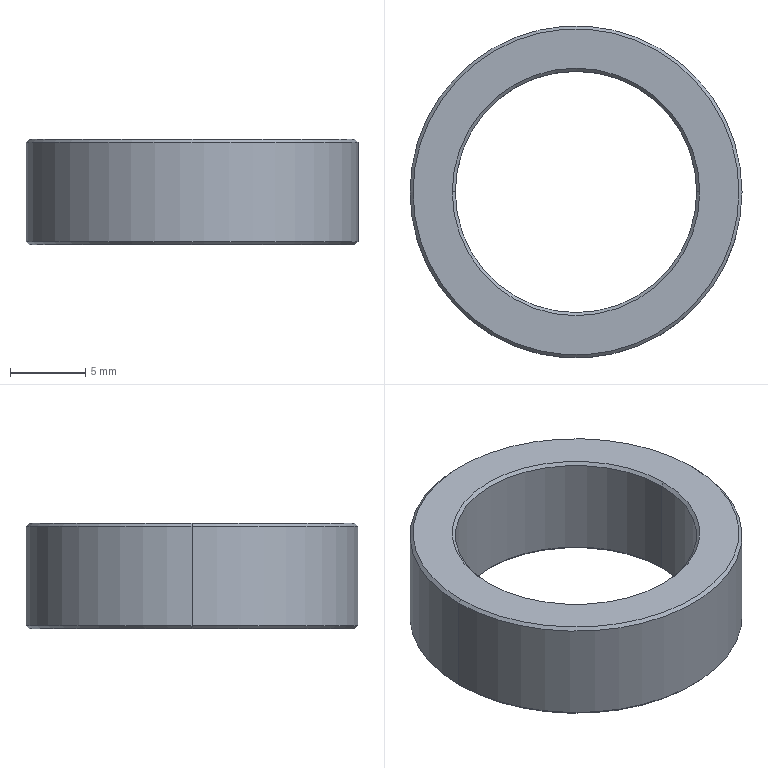Part | STEP file | BPSP-03-037Lift Retaining Ring_Default | 1 solid | 14 faces | box 22 x 22 x 7 mm | volume 1249 mm3 | cone 8 | cylinder 4 | plane 2 | commonest cylinder face diameters 16 x2 22 x2
STEP:
#1=CARTESIAN_POINT('',(0.,0.,0.));
#2=DIRECTION('',(0.,0.,1.));
#3=DIRECTION('',(1.,0.,0.));
#4=AXIS2_PLACEMENT_3D('',#1,#2,#3);
#5=CARTESIAN_POINT('',(10.8,0.,3.5));
#6=VERTEX_POINT('',#5);
#7=CARTESIAN_POINT('',(-10.8,0.,3.5));
#8=VERTEX_POINT('',#7);
#9=CARTESIAN_POINT('',(0.,0.,3.5));
#10=DIRECTION('',(0.,0.,1.));
#11=DIRECTION('',(1.,0.,0.));
#12=AXIS2_PLACEMENT_3D('',#9,#10,#11);
#13=CIRCLE('',#12,10.8);
#14=CARTESIAN_POINT('',(0.,0.,3.5));
#15=DIRECTION('',(0.,0.,-1.));
#16=DIRECTION('',(-1.,0.,0.));
#17=AXIS2_PLACEMENT_3D('',#14,#15,#16);
#18=CONICAL_SURFACE('',#17,10.8,0.7854);
#19=CARTESIAN_POINT('',(3.142,0.));
#20=DIRECTION('',(-1.,0.));
#21=VECTOR('',#20,1.);
#22=LINE('',#19,#21);
#23=(GEOMETRIC_REPRESENTATION_CONTEXT(2)PARAMETRIC_REPRESENTATION_CONTEXT()REPRESENTATION_CONTEXT('',''));
#24=DEFINITIONAL_REPRESENTATION('',(#22),#23);
#25=PCURVE('',#18,#24);
#26=CARTESIAN_POINT('',(0.,0.,3.5));
#27=DIRECTION('',(0.,0.,1.));
#28=DIRECTION('',(1.,0.,0.));
#29=AXIS2_PLACEMENT_3D('',#26,#27,#28);
#30=PLANE('',#29);
#31=CARTESIAN_POINT('',(0.,0.));
#32=DIRECTION('',(1.,0.));
#33=AXIS2_PLACEMENT_2D('',#31,#32);
#34=CIRCLE('',#33,10.8);
#35=(GEOMETRIC_REPRESENTATION_CONTEXT(2)PARAMETRIC_REPRESENTATION_CONTEXT()REPRESENTATION_CONTEXT('',''));
#36=DEFINITIONAL_REPRESENTATION('',(#34),#35);
#37=PCURVE('',#30,#36);
#38=SURFACE_CURVE('',#13,(#25,#37),.PCURVE_S1.);
#39=EDGE_CURVE('',#6,#8,#38,.T.);
#40=ORIENTED_EDGE('',*,*,#39,.F.);
#41=CARTESIAN_POINT('',(11.,0.,3.3));
#42=VERTEX_POINT('',#41);
#43=CARTESIAN_POINT('',(10.8,0.,3.5));
#44=DIRECTION('',(0.7071,0.,-0.7071));
#45=VECTOR('',#44,1.);
#46=LINE('',#43,#45);
#47=CARTESIAN_POINT('',(3.142,0.));
#48=DIRECTION('',(0.,1.));
#49=VECTOR('',#48,1.);
#50=LINE('',#47,#49);
#51=(GEOMETRIC_REPRESENTATION_CONTEXT(2)PARAMETRIC_REPRESENTATION_CONTEXT()REPRESENTATION_CONTEXT('',''));
#52=DEFINITIONAL_REPRESENTATION('',(#50),#51);
#53=PCURVE('',#18,#52);
#54=CARTESIAN_POINT('',(0.,0.,3.5));
#55=DIRECTION('',(0.,0.,-1.));
#56=DIRECTION('',(-1.,0.,0.));
#57=AXIS2_PLACEMENT_3D('',#54,#55,#56);
#58=CONICAL_SURFACE('',#57,10.8,0.7854);
#59=CARTESIAN_POINT('',(3.142,0.));
#60=DIRECTION('',(0.,1.));
#61=VECTOR('',#60,1.);
#62=LINE('',#59,#61);
#63=(GEOMETRIC_REPRESENTATION_CONTEXT(2)PARAMETRIC_REPRESENTATION_CONTEXT()REPRESENTATION_CONTEXT('',''));
#64=DEFINITIONAL_REPRESENTATION('',(#62),#63);
#65=PCURVE('',#58,#64);
#66=SURFACE_CURVE('',#46,(#53,#65),.PCURVE_S1.);
#67=EDGE_CURVE('',#6,#42,#66,.T.);
#68=ORIENTED_EDGE('',*,*,#67,.T.);
#69=CARTESIAN_POINT('',(-11.,0.,3.3));
#70=VERTEX_POINT('',#69);
#71=CARTESIAN_POINT('',(0.,0.,3.3));
#72=DIRECTION('',(0.,0.,-1.));
#73=DIRECTION('',(1.,0.,0.));
#74=AXIS2_PLACEMENT_3D('',#71,#72,#73);
#75=CIRCLE('',#74,11.);
#76=CARTESIAN_POINT('',(-3.142,0.2));
#77=DIRECTION('',(1.,0.));
#78=VECTOR('',#77,1.);
#79=LINE('',#76,#78);
#80=(GEOMETRIC_REPRESENTATION_CONTEXT(2)PARAMETRIC_REPRESENTATION_CONTEXT()REPRESENTATION_CONTEXT('',''));
#81=DEFINITIONAL_REPRESENTATION('',(#79),#80);
#82=PCURVE('',#18,#81);
#83=CARTESIAN_POINT('',(0.,0.,3.5));
#84=DIRECTION('',(0.,0.,-1.));
#85=DIRECTION('',(-1.,0.,0.));
#86=AXIS2_PLACEMENT_3D('',#83,#84,#85);
#87=CYLINDRICAL_SURFACE('',#86,11.);
#88=CARTESIAN_POINT('',(-3.142,0.2));
#89=DIRECTION('',(1.,0.));
#90=VECTOR('',#89,1.);
#91=LINE('',#88,#90);
#92=(GEOMETRIC_REPRESENTATION_CONTEXT(2)PARAMETRIC_REPRESENTATION_CONTEXT()REPRESENTATION_CONTEXT('',''));
#93=DEFINITIONAL_REPRESENTATION('',(#91),#92);
#94=PCURVE('',#87,#93);
#95=SURFACE_CURVE('',#75,(#82,#94),.PCURVE_S1.);
#96=EDGE_CURVE('',#70,#42,#95,.T.);
#97=ORIENTED_EDGE('',*,*,#96,.F.);
#98=CARTESIAN_POINT('',(-10.8,0.,3.5));
#99=DIRECTION('',(-0.7071,0.,-0.7071));
#100=VECTOR('',#99,1.);
#101=LINE('',#98,#100);
#102=CARTESIAN_POINT('',(0.,0.));
#103=DIRECTION('',(0.,1.));
#104=VECTOR('',#103,1.);
#105=LINE('',#102,#104);
#106=(GEOMETRIC_REPRESENTATION_CONTEXT(2)PARAMETRIC_REPRESENTATION_CONTEXT()REPRESENTATION_CONTEXT('',''));
#107=DEFINITIONAL_REPRESENTATION('',(#105),#106);
#108=PCURVE('',#18,#107);
#109=CARTESIAN_POINT('',(6.283,0.));
#110=DIRECTION('',(0.,1.));
#111=VECTOR('',#110,1.);
#112=LINE('',#109,#111);
#113=(GEOMETRIC_REPRESENTATION_CONTEXT(2)PARAMETRIC_REPRESENTATION_CONTEXT()REPRESENTATION_CONTEXT('',''));
#114=DEFINITIONAL_REPRESENTATION('',(#112),#113);
#115=PCURVE('',#58,#114);
#116=SURFACE_CURVE('',#101,(#108,#115),.PCURVE_S1.);
#117=EDGE_CURVE('',#8,#70,#116,.T.);
#118=ORIENTED_EDGE('',*,*,#117,.F.);
#119=EDGE_LOOP('',(#40,#68,#97,#118));
#120=FACE_BOUND('',#119,.T.);
#121=ADVANCED_FACE('',(#120),#18,.T.);
#122=CARTESIAN_POINT('',(8.,0.,3.3));
#123=VERTEX_POINT('',#122);
#124=CARTESIAN_POINT('',(8.2,0.,3.5));
#125=VERTEX_POINT('',#124);
#126=CARTESIAN_POINT('',(8.,0.,3.3));
#127=DIRECTION('',(0.7071,0.,0.7071));
#128=VECTOR('',#127,1.);
#129=LINE('',#126,#128);
#130=CARTESIAN_POINT('',(0.,0.,3.3));
#131=DIRECTION('',(0.,0.,1.));
#132=DIRECTION('',(1.,0.,0.));
#133=AXIS2_PLACEMENT_3D('',#130,#131,#132);
#134=CONICAL_SURFACE('',#133,8.,0.7854);
#135=CARTESIAN_POINT('',(6.283,0.));
#136=DIRECTION('',(0.,1.));
#137=VECTOR('',#136,1.);
#138=LINE('',#135,#137);
#139=(GEOMETRIC_REPRESENTATION_CONTEXT(2)PARAMETRIC_REPRESENTATION_CONTEXT()REPRESENTATION_CONTEXT('',''));
#140=DEFINITIONAL_REPRESENTATION('',(#138),#139);
#141=PCURVE('',#134,#140);
#142=CARTESIAN_POINT('',(0.,0.,3.3));
#143=DIRECTION('',(0.,0.,1.));
#144=DIRECTION('',(1.,0.,0.));
#145=AXIS2_PLACEMENT_3D('',#142,#143,#144);
#146=CONICAL_SURFACE('',#145,8.,0.7854);
#147=CARTESIAN_POINT('',(0.,0.));
#148=DIRECTION('',(0.,1.));
#149=VECTOR('',#148,1.);
#150=LINE('',#147,#149);
#151=(GEOMETRIC_REPRESENTATION_CONTEXT(2)PARAMETRIC_REPRESENTATION_CONTEXT()REPRESENTATION_CONTEXT('',''));
#152=DEFINITIONAL_REPRESENTATION('',(#150),#151);
#153=PCURVE('',#146,#152);
#154=SURFACE_CURVE('',#129,(#141,#153),.PCURVE_S1.);
#155=EDGE_CURVE('',#123,#125,#154,.T.);
#156=ORIENTED_EDGE('',*,*,#155,.T.);
#157=CARTESIAN_POINT('',(-8.2,0.,3.5));
#158=VERTEX_POINT('',#157);
#159=CARTESIAN_POINT('',(0.,0.,3.5));
#160=DIRECTION('',(0.,0.,-1.));
#161=DIRECTION('',(1.,0.,0.));
#162=AXIS2_PLACEMENT_3D('',#159,#160,#161);
#163=CIRCLE('',#162,8.2);
#164=CARTESIAN_POINT('',(6.283,0.2));
#165=DIRECTION('',(-1.,0.));
#166=VECTOR('',#165,1.);
#167=LINE('',#164,#166);
#168=(GEOMETRIC_REPRESENTATION_CONTEXT(2)PARAMETRIC_REPRESENTATION_CONTEXT()REPRESENTATION_CONTEXT('',''));
#169=DEFINITIONAL_REPRESENTATION('',(#167),#168);
#170=PCURVE('',#134,#169);
#171=CARTESIAN_POINT('',(8.2,0.));
#172=CARTESIAN_POINT('',(8.2,-14.203));
#173=CARTESIAN_POINT('',(-4.1,-7.101));
#174=CARTESIAN_POINT('',(-16.4,0.));
#175=CARTESIAN_POINT('',(-4.1,7.101));
#176=CARTESIAN_POINT('',(8.2,14.203));
#177=CARTESIAN_POINT('',(8.2,0.));
#178=(BOUNDED_CURVE()B_SPLINE_CURVE(2,(#171,#172,#173,#174,#175,#176,#177),.UNSPECIFIED.,.T.,.F.)B_SPLINE_CURVE_WITH_KNOTS((1,2,2,2,2,1),(-2.094,0.,2.094,4.189,6.283,8.378),.UNSPECIFIED.)CURVE()GEOMETRIC_REPRESENTATION_ITEM()RATIONAL_B_SPLINE_CURVE((1.,0.5,1.,0.5,1.,0.5,1.))REPRESENTATION_ITEM(''));
#179=(GEOMETRIC_REPRESENTATION_CONTEXT(2)PARAMETRIC_REPRESENTATION_CONTEXT()REPRESENTATION_CONTEXT('',''));
#180=DEFINITIONAL_REPRESENTATION('',(#178),#179);
#181=PCURVE('',#30,#180);
#182=SURFACE_CURVE('',#163,(#170,#181),.PCURVE_S1.);
#183=EDGE_CURVE('',#125,#158,#182,.T.);
#184=ORIENTED_EDGE('',*,*,#183,.T.);
#185=CARTESIAN_POINT('',(-8.,0.,3.3));
#186=VERTEX_POINT('',#185);
#187=CARTESIAN_POINT('',(-8.,0.,3.3));
#188=DIRECTION('',(-0.7071,0.,0.7071));
#189=VECTOR('',#188,1.);
#190=LINE('',#187,#189);
#191=CARTESIAN_POINT('',(3.142,0.));
#192=DIRECTION('',(0.,1.));
#193=VECTOR('',#192,1.);
#194=LINE('',#191,#193);
#195=(GEOMETRIC_REPRESENTATION_CONTEXT(2)PARAMETRIC_REPRESENTATION_CONTEXT()REPRESENTATION_CONTEXT('',''));
#196=DEFINITIONAL_REPRESENTATION('',(#194),#195);
#197=PCURVE('',#134,#196);
#198=CARTESIAN_POINT('',(3.142,0.));
#199=DIRECTION('',(0.,1.));
#200=VECTOR('',#199,1.);
#201=LINE('',#198,#200);
#202=(GEOMETRIC_REPRESENTATION_CONTEXT(2)PARAMETRIC_REPRESENTATION_CONTEXT()REPRESENTATION_CONTEXT('',''));
#203=DEFINITIONAL_REPRESENTATION('',(#201),#202);
#204=PCURVE('',#146,#203);
#205=SURFACE_CURVE('',#190,(#197,#204),.PCURVE_S1.);
#206=EDGE_CURVE('',#186,#158,#205,.T.);
#207=ORIENTED_EDGE('',*,*,#206,.F.);
#208=CARTESIAN_POINT('',(0.,0.,3.3));
#209=DIRECTION('',(0.,0.,1.));
#210=DIRECTION('',(1.,0.,0.));
#211=AXIS2_PLACEMENT_3D('',#208,#209,#210);
#212=CIRCLE('',#211,8.);
#213=CARTESIAN_POINT('',(0.,0.));
#214=DIRECTION('',(1.,0.));
#215=VECTOR('',#214,1.);
#216=LINE('',#213,#215);
#217=(GEOMETRIC_REPRESENTATION_CONTEXT(2)PARAMETRIC_REPRESENTATION_CONTEXT()REPRESENTATION_CONTEXT('',''));
#218=DEFINITIONAL_REPRESENTATION('',(#216),#217);
#219=PCURVE('',#134,#218);
#220=CARTESIAN_POINT('',(0.,0.,3.5));
#221=DIRECTION('',(0.,0.,-1.));
#222=DIRECTION('',(-1.,0.,0.));
#223=AXIS2_PLACEMENT_3D('',#220,#221,#222);
#224=CYLINDRICAL_SURFACE('',#223,8.);
#225=CARTESIAN_POINT('',(9.425,0.2));
#226=DIRECTION('',(-1.,0.));
#227=VECTOR('',#226,1.);
#228=LINE('',#225,#227);
#229=(GEOMETRIC_REPRESENTATION_CONTEXT(2)PARAMETRIC_REPRESENTATION_CONTEXT()REPRESENTATION_CONTEXT('',''));
#230=DEFINITIONAL_REPRESENTATION('',(#228),#229);
#231=PCURVE('',#224,#230);
#232=SURFACE_CURVE('',#212,(#219,#231),.PCURVE_S1.);
#233=EDGE_CURVE('',#186,#123,#232,.T.);
#234=ORIENTED_EDGE('',*,*,#233,.T.);
#235=EDGE_LOOP('',(#156,#184,#207,#234));
#236=FACE_BOUND('',#235,.F.);
#237=ADVANCED_FACE('',(#236),#134,.F.);
#238=CARTESIAN_POINT('',(-10.8,0.,-3.5));
#239=VERTEX_POINT('',#238);
#240=CARTESIAN_POINT('',(10.8,0.,-3.5));
#241=VERTEX_POINT('',#240);
#242=CARTESIAN_POINT('',(0.,0.,-3.5));
#243=DIRECTION('',(0.,0.,-1.));
#244=DIRECTION('',(1.,0.,0.));
#245=AXIS2_PLACEMENT_3D('',#242,#243,#244);
#246=CIRCLE('',#245,10.8);
#247=CARTESIAN_POINT('',(0.,0.,-3.3));
#248=DIRECTION('',(0.,0.,1.));
#249=DIRECTION('',(1.,0.,0.));
#250=AXIS2_PLACEMENT_3D('',#247,#248,#249);
#251=CONICAL_SURFACE('',#250,11.,0.7854);
#252=CARTESIAN_POINT('',(6.283,-0.2));
#253=DIRECTION('',(-1.,0.));
#254=VECTOR('',#253,1.);
#255=LINE('',#252,#254);
#256=(GEOMETRIC_REPRESENTATION_CONTEXT(2)PARAMETRIC_REPRESENTATION_CONTEXT()REPRESENTATION_CONTEXT('',''));
#257=DEFINITIONAL_REPRESENTATION('',(#255),#256);
#258=PCURVE('',#251,#257);
#259=CARTESIAN_POINT('',(0.,0.,-3.5));
#260=DIRECTION('',(0.,0.,1.));
#261=DIRECTION('',(1.,0.,0.));
#262=AXIS2_PLACEMENT_3D('',#259,#260,#261);
#263=PLANE('',#262);
#264=CARTESIAN_POINT('',(10.8,0.));
#265=CARTESIAN_POINT('',(10.8,-18.706));
#266=CARTESIAN_POINT('',(-5.4,-9.353));
#267=CARTESIAN_POINT('',(-21.6,0.));
#268=CARTESIAN_POINT('',(-5.4,9.353));
#269=CARTESIAN_POINT('',(10.8,18.706));
#270=CARTESIAN_POINT('',(10.8,0.));
#271=(BOUNDED_CURVE()B_SPLINE_CURVE(2,(#264,#265,#266,#267,#268,#269,#270),.UNSPECIFIED.,.T.,.F.)B_SPLINE_CURVE_WITH_KNOTS((1,2,2,2,2,1),(-2.094,0.,2.094,4.189,6.283,8.378),.UNSPECIFIED.)CURVE()GEOMETRIC_REPRESENTATION_ITEM()RATIONAL_B_SPLINE_CURVE((1.,0.5,1.,0.5,1.,0.5,1.))REPRESENTATION_ITEM(''));
#272=(GEOMETRIC_REPRESENTATION_CONTEXT(2)PARAMETRIC_REPRESENTATION_CONTEXT()REPRESENTATION_CONTEXT('',''));
#273=DEFINITIONAL_REPRESENTATION('',(#271),#272);
#274=PCURVE('',#263,#273);
#275=SURFACE_CURVE('',#246,(#258,#274),.PCURVE_S1.);
#276=EDGE_CURVE('',#239,#241,#275,.T.);
#277=ORIENTED_EDGE('',*,*,#276,.F.);
#278=CARTESIAN_POINT('',(-11.,0.,-3.3));
#279=VERTEX_POINT('',#278);
#280=CARTESIAN_POINT('',(-11.,0.,-3.3));
#281=DIRECTION('',(-0.7071,0.,0.7071));
#282=VECTOR('',#281,1.);
#283=LINE('',#280,#282);
#284=CARTESIAN_POINT('',(3.142,0.));
#285=DIRECTION('',(0.,1.));
#286=VECTOR('',#285,1.);
#287=LINE('',#284,#286);
#288=(GEOMETRIC_REPRESENTATION_CONTEXT(2)PARAMETRIC_REPRESENTATION_CONTEXT()REPRESENTATION_CONTEXT('',''));
#289=DEFINITIONAL_REPRESENTATION('',(#287),#288);
#290=PCURVE('',#251,#289);
#291=CARTESIAN_POINT('',(0.,0.,-3.3));
#292=DIRECTION('',(0.,0.,1.));
#293=DIRECTION('',(1.,0.,0.));
#294=AXIS2_PLACEMENT_3D('',#291,#292,#293);
#295=CONICAL_SURFACE('',#294,11.,0.7854);
#296=CARTESIAN_POINT('',(3.142,0.));
#297=DIRECTION('',(0.,1.));
#298=VECTOR('',#297,1.);
#299=LINE('',#296,#298);
#300=(GEOMETRIC_REPRESENTATION_CONTEXT(2)PARAMETRIC_REPRESENTATION_CONTEXT()REPRESENTATION_CONTEXT('',''));
#301=DEFINITIONAL_REPRESENTATION('',(#299),#300);
#302=PCURVE('',#295,#301);
#303=SURFACE_CURVE('',#283,(#290,#302),.PCURVE_S1.);
#304=EDGE_CURVE('',#239,#279,#303,.T.);
#305=ORIENTED_EDGE('',*,*,#304,.T.);
#306=CARTESIAN_POINT('',(11.,0.,-3.3));
#307=VERTEX_POINT('',#306);
#308=CARTESIAN_POINT('',(0.,0.,-3.3));
#309=DIRECTION('',(0.,0.,1.));
#310=DIRECTION('',(1.,0.,0.));
#311=AXIS2_PLACEMENT_3D('',#308,#309,#310);
#312=CIRCLE('',#311,11.);
#313=CARTESIAN_POINT('',(0.,0.));
#314=DIRECTION('',(1.,0.));
#315=VECTOR('',#314,1.);
#316=LINE('',#313,#315);
#317=(GEOMETRIC_REPRESENTATION_CONTEXT(2)PARAMETRIC_REPRESENTATION_CONTEXT()REPRESENTATION_CONTEXT('',''));
#318=DEFINITIONAL_REPRESENTATION('',(#316),#317);
#319=PCURVE('',#251,#318);
#320=CARTESIAN_POINT('',(3.142,6.8));
#321=DIRECTION('',(-1.,0.));
#322=VECTOR('',#321,1.);
#323=LINE('',#320,#322);
#324=(GEOMETRIC_REPRESENTATION_CONTEXT(2)PARAMETRIC_REPRESENTATION_CONTEXT()REPRESENTATION_CONTEXT('',''));
#325=DEFINITIONAL_REPRESENTATION('',(#323),#324);
#326=PCURVE('',#87,#325);
#327=SURFACE_CURVE('',#312,(#319,#326),.PCURVE_S1.);
#328=EDGE_CURVE('',#307,#279,#327,.T.);
#329=ORIENTED_EDGE('',*,*,#328,.F.);
#330=CARTESIAN_POINT('',(11.,0.,-3.3));
#331=DIRECTION('',(0.7071,0.,0.7071));
#332=VECTOR('',#331,1.);
#333=LINE('',#330,#332);
#334=CARTESIAN_POINT('',(0.,0.));
#335=DIRECTION('',(0.,1.));
#336=VECTOR('',#335,1.);
#337=LINE('',#334,#336);
#338=(GEOMETRIC_REPRESENTATION_CONTEXT(2)PARAMETRIC_REPRESENTATION_CONTEXT()REPRESENTATION_CONTEXT('',''));
#339=DEFINITIONAL_REPRESENTATION('',(#337),#338);
#340=PCURVE('',#251,#339);
#341=CARTESIAN_POINT('',(6.283,0.));
#342=DIRECTION('',(0.,1.));
#343=VECTOR('',#342,1.);
#344=LINE('',#341,#343);
#345=(GEOMETRIC_REPRESENTATION_CONTEXT(2)PARAMETRIC_REPRESENTATION_CONTEXT()REPRESENTATION_CONTEXT('',''));
#346=DEFINITIONAL_REPRESENTATION('',(#344),#345);
#347=PCURVE('',#295,#346);
#348=SURFACE_CURVE('',#333,(#340,#347),.PCURVE_S1.);
#349=EDGE_CURVE('',#241,#307,#348,.T.);
#350=ORIENTED_EDGE('',*,*,#349,.F.);
#351=EDGE_LOOP('',(#277,#305,#329,#350));
#352=FACE_BOUND('',#351,.T.);
#353=ADVANCED_FACE('',(#352),#251,.T.);
#354=CARTESIAN_POINT('',(-8.,0.,-3.3));
#355=VERTEX_POINT('',#354);
#356=CARTESIAN_POINT('',(-8.2,0.,-3.5));
#357=VERTEX_POINT('',#356);
#358=CARTESIAN_POINT('',(-8.2,0.,-3.5));
#359=DIRECTION('',(-0.7071,0.,-0.7071));
#360=VECTOR('',#359,1.);
#361=LINE('',#358,#360);
#362=CARTESIAN_POINT('',(0.,0.,-3.5));
#363=DIRECTION('',(0.,0.,-1.));
#364=DIRECTION('',(-1.,0.,0.));
#365=AXIS2_PLACEMENT_3D('',#362,#363,#364);
#366=CONICAL_SURFACE('',#365,8.2,0.7854);
#367=CARTESIAN_POINT('',(6.283,0.));
#368=DIRECTION('',(0.,1.));
#369=VECTOR('',#368,1.);
#370=LINE('',#367,#369);
#371=(GEOMETRIC_REPRESENTATION_CONTEXT(2)PARAMETRIC_REPRESENTATION_CONTEXT()REPRESENTATION_CONTEXT('',''));
#372=DEFINITIONAL_REPRESENTATION('',(#370),#371);
#373=PCURVE('',#366,#372);
#374=CARTESIAN_POINT('',(0.,0.,-3.5));
#375=DIRECTION('',(0.,0.,-1.));
#376=DIRECTION('',(-1.,0.,0.));
#377=AXIS2_PLACEMENT_3D('',#374,#375,#376);
#378=CONICAL_SURFACE('',#377,8.2,0.7854);
#379=CARTESIAN_POINT('',(0.,0.));
#380=DIRECTION('',(0.,1.));
#381=VECTOR('',#380,1.);
#382=LINE('',#379,#381);
#383=(GEOMETRIC_REPRESENTATION_CONTEXT(2)PARAMETRIC_REPRESENTATION_CONTEXT()REPRESENTATION_CONTEXT('',''));
#384=DEFINITIONAL_REPRESENTATION('',(#382),#383);
#385=PCURVE('',#378,#384);
#386=SURFACE_CURVE('',#361,(#373,#385),.PCURVE_S1.);
#387=EDGE_CURVE('',#355,#357,#386,.T.);
#388=ORIENTED_EDGE('',*,*,#387,.T.);
#389=CARTESIAN_POINT('',(8.2,0.,-3.5));
#390=VERTEX_POINT('',#389);
#391=CARTESIAN_POINT('',(0.,0.,-3.5));
#392=DIRECTION('',(0.,0.,1.));
#393=DIRECTION('',(1.,0.,0.));
#394=AXIS2_PLACEMENT_3D('',#391,#392,#393);
#395=CIRCLE('',#394,8.2);
#396=CARTESIAN_POINT('',(9.425,0.));
#397=DIRECTION('',(-1.,0.));
#398=VECTOR('',#397,1.);
#399=LINE('',#396,#398);
#400=(GEOMETRIC_REPRESENTATION_CONTEXT(2)PARAMETRIC_REPRESENTATION_CONTEXT()REPRESENTATION_CONTEXT('',''));
#401=DEFINITIONAL_REPRESENTATION('',(#399),#400);
#402=PCURVE('',#366,#401);
#403=CARTESIAN_POINT('',(0.,0.));
#404=DIRECTION('',(1.,0.));
#405=AXIS2_PLACEMENT_2D('',#403,#404);
#406=CIRCLE('',#405,8.2);
#407=(GEOMETRIC_REPRESENTATION_CONTEXT(2)PARAMETRIC_REPRESENTATION_CONTEXT()REPRESENTATION_CONTEXT('',''));
#408=DEFINITIONAL_REPRESENTATION('',(#406),#407);
#409=PCURVE('',#263,#408);
#410=SURFACE_CURVE('',#395,(#402,#409),.PCURVE_S1.);
#411=EDGE_CURVE('',#357,#390,#410,.T.);
#412=ORIENTED_EDGE('',*,*,#411,.T.);
#413=CARTESIAN_POINT('',(8.,0.,-3.3));
#414=VERTEX_POINT('',#413);
#415=CARTESIAN_POINT('',(8.2,0.,-3.5));
#416=DIRECTION('',(0.7071,0.,-0.7071));
#417=VECTOR('',#416,1.);
#418=LINE('',#415,#417);
#419=CARTESIAN_POINT('',(3.142,0.));
#420=DIRECTION('',(0.,1.));
#421=VECTOR('',#420,1.);
#422=LINE('',#419,#421);
#423=(GEOMETRIC_REPRESENTATION_CONTEXT(2)PARAMETRIC_REPRESENTATION_CONTEXT()REPRESENTATION_CONTEXT('',''));
#424=DEFINITIONAL_REPRESENTATION('',(#422),#423);
#425=PCURVE('',#366,#424);
#426=CARTESIAN_POINT('',(3.142,0.));
#427=DIRECTION('',(0.,1.));
#428=VECTOR('',#427,1.);
#429=LINE('',#426,#428);
#430=(GEOMETRIC_REPRESENTATION_CONTEXT(2)PARAMETRIC_REPRESENTATION_CONTEXT()REPRESENTATION_CONTEXT('',''));
#431=DEFINITIONAL_REPRESENTATION('',(#429),#430);
#432=PCURVE('',#378,#431);
#433=SURFACE_CURVE('',#418,(#425,#432),.PCURVE_S1.);
#434=EDGE_CURVE('',#414,#390,#433,.T.);
#435=ORIENTED_EDGE('',*,*,#434,.F.);
#436=CARTESIAN_POINT('',(0.,0.,-3.3));
#437=DIRECTION('',(0.,0.,-1.));
#438=DIRECTION('',(1.,0.,0.));
#439=AXIS2_PLACEMENT_3D('',#436,#437,#438);
#440=CIRCLE('',#439,8.);
#441=CARTESIAN_POINT('',(3.142,-0.2));
#442=DIRECTION('',(1.,0.));
#443=VECTOR('',#442,1.);
#444=LINE('',#441,#443);
#445=(GEOMETRIC_REPRESENTATION_CONTEXT(2)PARAMETRIC_REPRESENTATION_CONTEXT()REPRESENTATION_CONTEXT('',''));
#446=DEFINITIONAL_REPRESENTATION('',(#444),#445);
#447=PCURVE('',#366,#446);
#448=CARTESIAN_POINT('',(3.142,6.8));
#449=DIRECTION('',(1.,0.));
#450=VECTOR('',#449,1.);
#451=LINE('',#448,#450);
#452=(GEOMETRIC_REPRESENTATION_CONTEXT(2)PARAMETRIC_REPRESENTATION_CONTEXT()REPRESENTATION_CONTEXT('',''));
#453=DEFINITIONAL_REPRESENTATION('',(#451),#452);
#454=PCURVE('',#224,#453);
#455=SURFACE_CURVE('',#440,(#447,#454),.PCURVE_S1.);
#456=EDGE_CURVE('',#414,#355,#455,.T.);
#457=ORIENTED_EDGE('',*,*,#456,.T.);
#458=EDGE_LOOP('',(#388,#412,#435,#457));
#459=FACE_BOUND('',#458,.F.);
#460=ADVANCED_FACE('',(#459),#366,.F.);
#461=CARTESIAN_POINT('',(-8.,0.,3.5));
#462=DIRECTION('',(0.,0.,-1.));
#463=VECTOR('',#462,1.);
#464=LINE('',#461,#463);
#465=CARTESIAN_POINT('',(6.283,0.));
#466=DIRECTION('',(0.,1.));
#467=VECTOR('',#466,1.);
#468=LINE('',#465,#467);
#469=(GEOMETRIC_REPRESENTATION_CONTEXT(2)PARAMETRIC_REPRESENTATION_CONTEXT()REPRESENTATION_CONTEXT('',''));
#470=DEFINITIONAL_REPRESENTATION('',(#468),#469);
#471=PCURVE('',#224,#470);
#472=CARTESIAN_POINT('',(0.,0.,3.5));
#473=DIRECTION('',(0.,0.,-1.));
#474=DIRECTION('',(-1.,0.,0.));
#475=AXIS2_PLACEMENT_3D('',#472,#473,#474);
#476=CYLINDRICAL_SURFACE('',#475,8.);
#477=CARTESIAN_POINT('',(0.,0.));
#478=DIRECTION('',(0.,1.));
#479=VECTOR('',#478,1.);
#480=LINE('',#477,#479);
#481=(GEOMETRIC_REPRESENTATION_CONTEXT(2)PARAMETRIC_REPRESENTATION_CONTEXT()REPRESENTATION_CONTEXT('',''));
#482=DEFINITIONAL_REPRESENTATION('',(#480),#481);
#483=PCURVE('',#476,#482);
#484=SURFACE_CURVE('',#464,(#471,#483),.PCURVE_S1.);
#485=EDGE_CURVE('',#186,#355,#484,.T.);
#486=ORIENTED_EDGE('',*,*,#485,.T.);
#487=ORIENTED_EDGE('',*,*,#456,.F.);
#488=CARTESIAN_POINT('',(8.,0.,3.5));
#489=DIRECTION('',(0.,0.,-1.));
#490=VECTOR('',#489,1.);
#491=LINE('',#488,#490);
#492=CARTESIAN_POINT('',(3.142,0.));
#493=DIRECTION('',(0.,1.));
#494=VECTOR('',#493,1.);
#495=LINE('',#492,#494);
#496=(GEOMETRIC_REPRESENTATION_CONTEXT(2)PARAMETRIC_REPRESENTATION_CONTEXT()REPRESENTATION_CONTEXT('',''));
#497=DEFINITIONAL_REPRESENTATION('',(#495),#496);
#498=PCURVE('',#224,#497);
#499=CARTESIAN_POINT('',(3.142,0.));
#500=DIRECTION('',(0.,1.));
#501=VECTOR('',#500,1.);
#502=LINE('',#499,#501);
#503=(GEOMETRIC_REPRESENTATION_CONTEXT(2)PARAMETRIC_REPRESENTATION_CONTEXT()REPRESENTATION_CONTEXT('',''));
#504=DEFINITIONAL_REPRESENTATION('',(#502),#503);
#505=PCURVE('',#476,#504);
#506=SURFACE_CURVE('',#491,(#498,#505),.PCURVE_S1.);
#507=EDGE_CURVE('',#123,#414,#506,.T.);
#508=ORIENTED_EDGE('',*,*,#507,.F.);
#509=ORIENTED_EDGE('',*,*,#233,.F.);
#510=EDGE_LOOP('',(#486,#487,#508,#509));
#511=FACE_BOUND('',#510,.F.);
#512=ADVANCED_FACE('',(#511),#224,.F.);
#513=ORIENTED_EDGE('',*,*,#96,.T.);
#514=CARTESIAN_POINT('',(11.,0.,3.5));
#515=DIRECTION('',(0.,0.,-1.));
#516=VECTOR('',#515,1.);
#517=LINE('',#514,#516);
#518=CARTESIAN_POINT('',(3.142,0.));
#519=DIRECTION('',(0.,1.));
#520=VECTOR('',#519,1.);
#521=LINE('',#518,#520);
#522=(GEOMETRIC_REPRESENTATION_CONTEXT(2)PARAMETRIC_REPRESENTATION_CONTEXT()REPRESENTATION_CONTEXT('',''));
#523=DEFINITIONAL_REPRESENTATION('',(#521),#522);
#524=PCURVE('',#87,#523);
#525=CARTESIAN_POINT('',(0.,0.,3.5));
#526=DIRECTION('',(0.,0.,-1.));
#527=DIRECTION('',(-1.,0.,0.));
#528=AXIS2_PLACEMENT_3D('',#525,#526,#527);
#529=CYLINDRICAL_SURFACE('',#528,11.);
#530=CARTESIAN_POINT('',(3.142,0.));
#531=DIRECTION('',(0.,1.));
#532=VECTOR('',#531,1.);
#533=LINE('',#530,#532);
#534=(GEOMETRIC_REPRESENTATION_CONTEXT(2)PARAMETRIC_REPRESENTATION_CONTEXT()REPRESENTATION_CONTEXT('',''));
#535=DEFINITIONAL_REPRESENTATION('',(#533),#534);
#536=PCURVE('',#529,#535);
#537=SURFACE_CURVE('',#517,(#524,#536),.PCURVE_S1.);
#538=EDGE_CURVE('',#42,#307,#537,.T.);
#539=ORIENTED_EDGE('',*,*,#538,.T.);
#540=ORIENTED_EDGE('',*,*,#328,.T.);
#541=CARTESIAN_POINT('',(-11.,0.,3.5));
#542=DIRECTION('',(0.,0.,-1.));
#543=VECTOR('',#542,1.);
#544=LINE('',#541,#543);
#545=CARTESIAN_POINT('',(0.,0.));
#546=DIRECTION('',(0.,1.));
#547=VECTOR('',#546,1.);
#548=LINE('',#545,#547);
#549=(GEOMETRIC_REPRESENTATION_CONTEXT(2)PARAMETRIC_REPRESENTATION_CONTEXT()REPRESENTATION_CONTEXT('',''));
#550=DEFINITIONAL_REPRESENTATION('',(#548),#549);
#551=PCURVE('',#87,#550);
#552=CARTESIAN_POINT('',(6.283,0.));
#553=DIRECTION('',(0.,1.));
#554=VECTOR('',#553,1.);
#555=LINE('',#552,#554);
#556=(GEOMETRIC_REPRESENTATION_CONTEXT(2)PARAMETRIC_REPRESENTATION_CONTEXT()REPRESENTATION_CONTEXT('',''));
#557=DEFINITIONAL_REPRESENTATION('',(#555),#556);
#558=PCURVE('',#529,#557);
#559=SURFACE_CURVE('',#544,(#551,#558),.PCURVE_S1.);
#560=EDGE_CURVE('',#70,#279,#559,.T.);
#561=ORIENTED_EDGE('',*,*,#560,.F.);
#562=EDGE_LOOP('',(#513,#539,#540,#561));
#563=FACE_BOUND('',#562,.T.);
#564=ADVANCED_FACE('',(#563),#87,.T.);
#565=ORIENTED_EDGE('',*,*,#183,.T.);
#566=CARTESIAN_POINT('',(0.,0.,3.5));
#567=DIRECTION('',(0.,0.,-1.));
#568=DIRECTION('',(1.,0.,0.));
#569=AXIS2_PLACEMENT_3D('',#566,#567,#568);
#570=CIRCLE('',#569,8.2);
#571=CARTESIAN_POINT('',(8.2,0.));
#572=CARTESIAN_POINT('',(8.2,-14.203));
#573=CARTESIAN_POINT('',(-4.1,-7.101));
#574=CARTESIAN_POINT('',(-16.4,0.));
#575=CARTESIAN_POINT('',(-4.1,7.101));
#576=CARTESIAN_POINT('',(8.2,14.203));
#577=CARTESIAN_POINT('',(8.2,0.));
#578=(BOUNDED_CURVE()B_SPLINE_CURVE(2,(#571,#572,#573,#574,#575,#576,#577),.UNSPECIFIED.,.T.,.F.)B_SPLINE_CURVE_WITH_KNOTS((1,2,2,2,2,1),(-2.094,0.,2.094,4.189,6.283,8.378),.UNSPECIFIED.)CURVE()GEOMETRIC_REPRESENTATION_ITEM()RATIONAL_B_SPLINE_CURVE((1.,0.5,1.,0.5,1.,0.5,1.))REPRESENTATION_ITEM(''));
#579=(GEOMETRIC_REPRESENTATION_CONTEXT(2)PARAMETRIC_REPRESENTATION_CONTEXT()REPRESENTATION_CONTEXT('',''));
#580=DEFINITIONAL_REPRESENTATION('',(#578),#579);
#581=PCURVE('',#30,#580);
#582=CARTESIAN_POINT('',(6.283,0.2));
#583=DIRECTION('',(-1.,0.));
#584=VECTOR('',#583,1.);
#585=LINE('',#582,#584);
#586=(GEOMETRIC_REPRESENTATION_CONTEXT(2)PARAMETRIC_REPRESENTATION_CONTEXT()REPRESENTATION_CONTEXT('',''));
#587=DEFINITIONAL_REPRESENTATION('',(#585),#586);
#588=PCURVE('',#146,#587);
#589=SURFACE_CURVE('',#570,(#581,#588),.PCURVE_S1.);
#590=EDGE_CURVE('',#158,#125,#589,.T.);
#591=ORIENTED_EDGE('',*,*,#590,.T.);
#592=EDGE_LOOP('',(#565,#591));
#593=FACE_BOUND('',#592,.T.);
#594=CARTESIAN_POINT('',(0.,0.,3.5));
#595=DIRECTION('',(0.,0.,1.));
#596=DIRECTION('',(1.,0.,0.));
#597=AXIS2_PLACEMENT_3D('',#594,#595,#596);
#598=CIRCLE('',#597,10.8);
#599=CARTESIAN_POINT('',(0.,0.));
#600=DIRECTION('',(1.,0.));
#601=AXIS2_PLACEMENT_2D('',#599,#600);
#602=CIRCLE('',#601,10.8);
#603=(GEOMETRIC_REPRESENTATION_CONTEXT(2)PARAMETRIC_REPRESENTATION_CONTEXT()REPRESENTATION_CONTEXT('',''));
#604=DEFINITIONAL_REPRESENTATION('',(#602),#603);
#605=PCURVE('',#30,#604);
#606=CARTESIAN_POINT('',(9.425,0.));
#607=DIRECTION('',(-1.,0.));
#608=VECTOR('',#607,1.);
#609=LINE('',#606,#608);
#610=(GEOMETRIC_REPRESENTATION_CONTEXT(2)PARAMETRIC_REPRESENTATION_CONTEXT()REPRESENTATION_CONTEXT('',''));
#611=DEFINITIONAL_REPRESENTATION('',(#609),#610);
#612=PCURVE('',#58,#611);
#613=SURFACE_CURVE('',#598,(#605,#612),.PCURVE_S1.);
#614=EDGE_CURVE('',#8,#6,#613,.T.);
#615=ORIENTED_EDGE('',*,*,#614,.T.);
#616=ORIENTED_EDGE('',*,*,#39,.T.);
#617=EDGE_LOOP('',(#615,#616));
#618=FACE_BOUND('',#617,.T.);
#619=ADVANCED_FACE('',(#593,#618),#30,.T.);
#620=ORIENTED_EDGE('',*,*,#411,.T.);
#621=CARTESIAN_POINT('',(0.,0.,-3.5));
#622=DIRECTION('',(0.,0.,1.));
#623=DIRECTION('',(1.,0.,0.));
#624=AXIS2_PLACEMENT_3D('',#621,#622,#623);
#625=CIRCLE('',#624,8.2);
#626=CARTESIAN_POINT('',(0.,0.));
#627=DIRECTION('',(1.,0.));
#628=AXIS2_PLACEMENT_2D('',#626,#627);
#629=CIRCLE('',#628,8.2);
#630=(GEOMETRIC_REPRESENTATION_CONTEXT(2)PARAMETRIC_REPRESENTATION_CONTEXT()REPRESENTATION_CONTEXT('',''));
#631=DEFINITIONAL_REPRESENTATION('',(#629),#630);
#632=PCURVE('',#263,#631);
#633=CARTESIAN_POINT('',(3.142,0.));
#634=DIRECTION('',(-1.,0.));
#635=VECTOR('',#634,1.);
#636=LINE('',#633,#635);
#637=(GEOMETRIC_REPRESENTATION_CONTEXT(2)PARAMETRIC_REPRESENTATION_CONTEXT()REPRESENTATION_CONTEXT('',''));
#638=DEFINITIONAL_REPRESENTATION('',(#636),#637);
#639=PCURVE('',#378,#638);
#640=SURFACE_CURVE('',#625,(#632,#639),.PCURVE_S1.);
#641=EDGE_CURVE('',#390,#357,#640,.T.);
#642=ORIENTED_EDGE('',*,*,#641,.T.);
#643=EDGE_LOOP('',(#620,#642));
#644=FACE_BOUND('',#643,.T.);
#645=CARTESIAN_POINT('',(0.,0.,-3.5));
#646=DIRECTION('',(0.,0.,-1.));
#647=DIRECTION('',(1.,0.,0.));
#648=AXIS2_PLACEMENT_3D('',#645,#646,#647);
#649=CIRCLE('',#648,10.8);
#650=CARTESIAN_POINT('',(10.8,0.));
#651=CARTESIAN_POINT('',(10.8,-18.706));
#652=CARTESIAN_POINT('',(-5.4,-9.353));
#653=CARTESIAN_POINT('',(-21.6,0.));
#654=CARTESIAN_POINT('',(-5.4,9.353));
#655=CARTESIAN_POINT('',(10.8,18.706));
#656=CARTESIAN_POINT('',(10.8,0.));
#657=(BOUNDED_CURVE()B_SPLINE_CURVE(2,(#650,#651,#652,#653,#654,#655,#656),.UNSPECIFIED.,.T.,.F.)B_SPLINE_CURVE_WITH_KNOTS((1,2,2,2,2,1),(-2.094,0.,2.094,4.189,6.283,8.378),.UNSPECIFIED.)CURVE()GEOMETRIC_REPRESENTATION_ITEM()RATIONAL_B_SPLINE_CURVE((1.,0.5,1.,0.5,1.,0.5,1.))REPRESENTATION_ITEM(''));
#658=(GEOMETRIC_REPRESENTATION_CONTEXT(2)PARAMETRIC_REPRESENTATION_CONTEXT()REPRESENTATION_CONTEXT('',''));
#659=DEFINITIONAL_REPRESENTATION('',(#657),#658);
#660=PCURVE('',#263,#659);
#661=CARTESIAN_POINT('',(6.283,-0.2));
#662=DIRECTION('',(-1.,0.));
#663=VECTOR('',#662,1.);
#664=LINE('',#661,#663);
#665=(GEOMETRIC_REPRESENTATION_CONTEXT(2)PARAMETRIC_REPRESENTATION_CONTEXT()REPRESENTATION_CONTEXT('',''));
#666=DEFINITIONAL_REPRESENTATION('',(#664),#665);
#667=PCURVE('',#295,#666);
#668=SURFACE_CURVE('',#649,(#660,#667),.PCURVE_S1.);
#669=EDGE_CURVE('',#241,#239,#668,.T.);
#670=ORIENTED_EDGE('',*,*,#669,.T.);
#671=ORIENTED_EDGE('',*,*,#276,.T.);
#672=EDGE_LOOP('',(#670,#671));
#673=FACE_BOUND('',#672,.T.);
#674=ADVANCED_FACE('',(#644,#673),#263,.F.);
#675=ORIENTED_EDGE('',*,*,#538,.F.);
#676=CARTESIAN_POINT('',(0.,0.,3.3));
#677=DIRECTION('',(0.,0.,-1.));
#678=DIRECTION('',(1.,0.,0.));
#679=AXIS2_PLACEMENT_3D('',#676,#677,#678);
#680=CIRCLE('',#679,11.);
#681=CARTESIAN_POINT('',(3.142,0.2));
#682=DIRECTION('',(1.,0.));
#683=VECTOR('',#682,1.);
#684=LINE('',#681,#683);
#685=(GEOMETRIC_REPRESENTATION_CONTEXT(2)PARAMETRIC_REPRESENTATION_CONTEXT()REPRESENTATION_CONTEXT('',''));
#686=DEFINITIONAL_REPRESENTATION('',(#684),#685);
#687=PCURVE('',#529,#686);
#688=CARTESIAN_POINT('',(3.142,0.2));
#689=DIRECTION('',(1.,0.));
#690=VECTOR('',#689,1.);
#691=LINE('',#688,#690);
#692=(GEOMETRIC_REPRESENTATION_CONTEXT(2)PARAMETRIC_REPRESENTATION_CONTEXT()REPRESENTATION_CONTEXT('',''));
#693=DEFINITIONAL_REPRESENTATION('',(#691),#692);
#694=PCURVE('',#58,#693);
#695=SURFACE_CURVE('',#680,(#687,#694),.PCURVE_S1.);
#696=EDGE_CURVE('',#42,#70,#695,.T.);
#697=ORIENTED_EDGE('',*,*,#696,.T.);
#698=ORIENTED_EDGE('',*,*,#560,.T.);
#699=CARTESIAN_POINT('',(0.,0.,-3.3));
#700=DIRECTION('',(0.,0.,1.));
#701=DIRECTION('',(1.,0.,0.));
#702=AXIS2_PLACEMENT_3D('',#699,#700,#701);
#703=CIRCLE('',#702,11.);
#704=CARTESIAN_POINT('',(9.425,6.8));
#705=DIRECTION('',(-1.,0.));
#706=VECTOR('',#705,1.);
#707=LINE('',#704,#706);
#708=(GEOMETRIC_REPRESENTATION_CONTEXT(2)PARAMETRIC_REPRESENTATION_CONTEXT()REPRESENTATION_CONTEXT('',''));
#709=DEFINITIONAL_REPRESENTATION('',(#707),#708);
#710=PCURVE('',#529,#709);
#711=CARTESIAN_POINT('',(0.,0.));
#712=DIRECTION('',(1.,0.));
#713=VECTOR('',#712,1.);
#714=LINE('',#711,#713);
#715=(GEOMETRIC_REPRESENTATION_CONTEXT(2)PARAMETRIC_REPRESENTATION_CONTEXT()REPRESENTATION_CONTEXT('',''));
#716=DEFINITIONAL_REPRESENTATION('',(#714),#715);
#717=PCURVE('',#295,#716);
#718=SURFACE_CURVE('',#703,(#710,#717),.PCURVE_S1.);
#719=EDGE_CURVE('',#279,#307,#718,.T.);
#720=ORIENTED_EDGE('',*,*,#719,.T.);
#721=EDGE_LOOP('',(#675,#697,#698,#720));
#722=FACE_BOUND('',#721,.T.);
#723=ADVANCED_FACE('',(#722),#529,.T.);
#724=CARTESIAN_POINT('',(0.,0.,-3.3));
#725=DIRECTION('',(0.,0.,-1.));
#726=DIRECTION('',(1.,0.,0.));
#727=AXIS2_PLACEMENT_3D('',#724,#725,#726);
#728=CIRCLE('',#727,8.);
#729=CARTESIAN_POINT('',(-3.142,6.8));
#730=DIRECTION('',(1.,0.));
#731=VECTOR('',#730,1.);
#732=LINE('',#729,#731);
#733=(GEOMETRIC_REPRESENTATION_CONTEXT(2)PARAMETRIC_REPRESENTATION_CONTEXT()REPRESENTATION_CONTEXT('',''));
#734=DEFINITIONAL_REPRESENTATION('',(#732),#733);
#735=PCURVE('',#476,#734);
#736=CARTESIAN_POINT('',(-3.142,-0.2));
#737=DIRECTION('',(1.,0.));
#738=VECTOR('',#737,1.);
#739=LINE('',#736,#738);
#740=(GEOMETRIC_REPRESENTATION_CONTEXT(2)PARAMETRIC_REPRESENTATION_CONTEXT()REPRESENTATION_CONTEXT('',''));
#741=DEFINITIONAL_REPRESENTATION('',(#739),#740);
#742=PCURVE('',#378,#741);
#743=SURFACE_CURVE('',#728,(#735,#742),.PCURVE_S1.);
#744=EDGE_CURVE('',#355,#414,#743,.T.);
#745=ORIENTED_EDGE('',*,*,#744,.F.);
#746=ORIENTED_EDGE('',*,*,#485,.F.);
#747=CARTESIAN_POINT('',(0.,0.,3.3));
#748=DIRECTION('',(0.,0.,1.));
#749=DIRECTION('',(1.,0.,0.));
#750=AXIS2_PLACEMENT_3D('',#747,#748,#749);
#751=CIRCLE('',#750,8.);
#752=CARTESIAN_POINT('',(3.142,0.2));
#753=DIRECTION('',(-1.,0.));
#754=VECTOR('',#753,1.);
#755=LINE('',#752,#754);
#756=(GEOMETRIC_REPRESENTATION_CONTEXT(2)PARAMETRIC_REPRESENTATION_CONTEXT()REPRESENTATION_CONTEXT('',''));
#757=DEFINITIONAL_REPRESENTATION('',(#755),#756);
#758=PCURVE('',#476,#757);
#759=CARTESIAN_POINT('',(0.,0.));
#760=DIRECTION('',(1.,0.));
#761=VECTOR('',#760,1.);
#762=LINE('',#759,#761);
#763=(GEOMETRIC_REPRESENTATION_CONTEXT(2)PARAMETRIC_REPRESENTATION_CONTEXT()REPRESENTATION_CONTEXT('',''));
#764=DEFINITIONAL_REPRESENTATION('',(#762),#763);
#765=PCURVE('',#146,#764);
#766=SURFACE_CURVE('',#751,(#758,#765),.PCURVE_S1.);
#767=EDGE_CURVE('',#123,#186,#766,.T.);
#768=ORIENTED_EDGE('',*,*,#767,.F.);
#769=ORIENTED_EDGE('',*,*,#507,.T.);
#770=EDGE_LOOP('',(#745,#746,#768,#769));
#771=FACE_BOUND('',#770,.F.);
#772=ADVANCED_FACE('',(#771),#476,.F.);
#773=ORIENTED_EDGE('',*,*,#641,.T.);
#774=ORIENTED_EDGE('',*,*,#387,.F.);
#775=ORIENTED_EDGE('',*,*,#744,.T.);
#776=ORIENTED_EDGE('',*,*,#434,.T.);
#777=EDGE_LOOP('',(#773,#774,#775,#776));
#778=FACE_BOUND('',#777,.F.);
#779=ADVANCED_FACE('',(#778),#378,.F.);
#780=ORIENTED_EDGE('',*,*,#304,.F.);
#781=ORIENTED_EDGE('',*,*,#669,.F.);
#782=ORIENTED_EDGE('',*,*,#349,.T.);
#783=ORIENTED_EDGE('',*,*,#719,.F.);
#784=EDGE_LOOP('',(#780,#781,#782,#783));
#785=FACE_BOUND('',#784,.T.);
#786=ADVANCED_FACE('',(#785),#295,.T.);
#787=ORIENTED_EDGE('',*,*,#590,.T.);
#788=ORIENTED_EDGE('',*,*,#155,.F.);
#789=ORIENTED_EDGE('',*,*,#767,.T.);
#790=ORIENTED_EDGE('',*,*,#206,.T.);
#791=EDGE_LOOP('',(#787,#788,#789,#790));
#792=FACE_BOUND('',#791,.F.);
#793=ADVANCED_FACE('',(#792),#146,.F.);
#794=ORIENTED_EDGE('',*,*,#67,.F.);
#795=ORIENTED_EDGE('',*,*,#614,.F.);
#796=ORIENTED_EDGE('',*,*,#117,.T.);
#797=ORIENTED_EDGE('',*,*,#696,.F.);
#798=EDGE_LOOP('',(#794,#795,#796,#797));
#799=FACE_BOUND('',#798,.T.);
#800=ADVANCED_FACE('',(#799),#58,.T.);
#801=CLOSED_SHELL('',(#121,#237,#353,#460,#512,#564,#619,#674,#723,#772,#779,#786,#793,#800));
#802=MANIFOLD_SOLID_BREP('',#801);
#803=(LENGTH_UNIT()NAMED_UNIT(*)SI_UNIT(.MILLI.,.METRE.));
#804=UNCERTAINTY_MEASURE_WITH_UNIT(LENGTH_MEASURE(0.0000001),#803,'','');
#805=(NAMED_UNIT(*)PLANE_ANGLE_UNIT()SI_UNIT($,.RADIAN.));
#806=(NAMED_UNIT(*)SI_UNIT($,.STERADIAN.)SOLID_ANGLE_UNIT());
#807=(GEOMETRIC_REPRESENTATION_CONTEXT(3)GLOBAL_UNCERTAINTY_ASSIGNED_CONTEXT((#804))GLOBAL_UNIT_ASSIGNED_CONTEXT((#803,#805,#806))REPRESENTATION_CONTEXT('',''));
#808=ADVANCED_BREP_SHAPE_REPRESENTATION('',(#4,#802),#807);